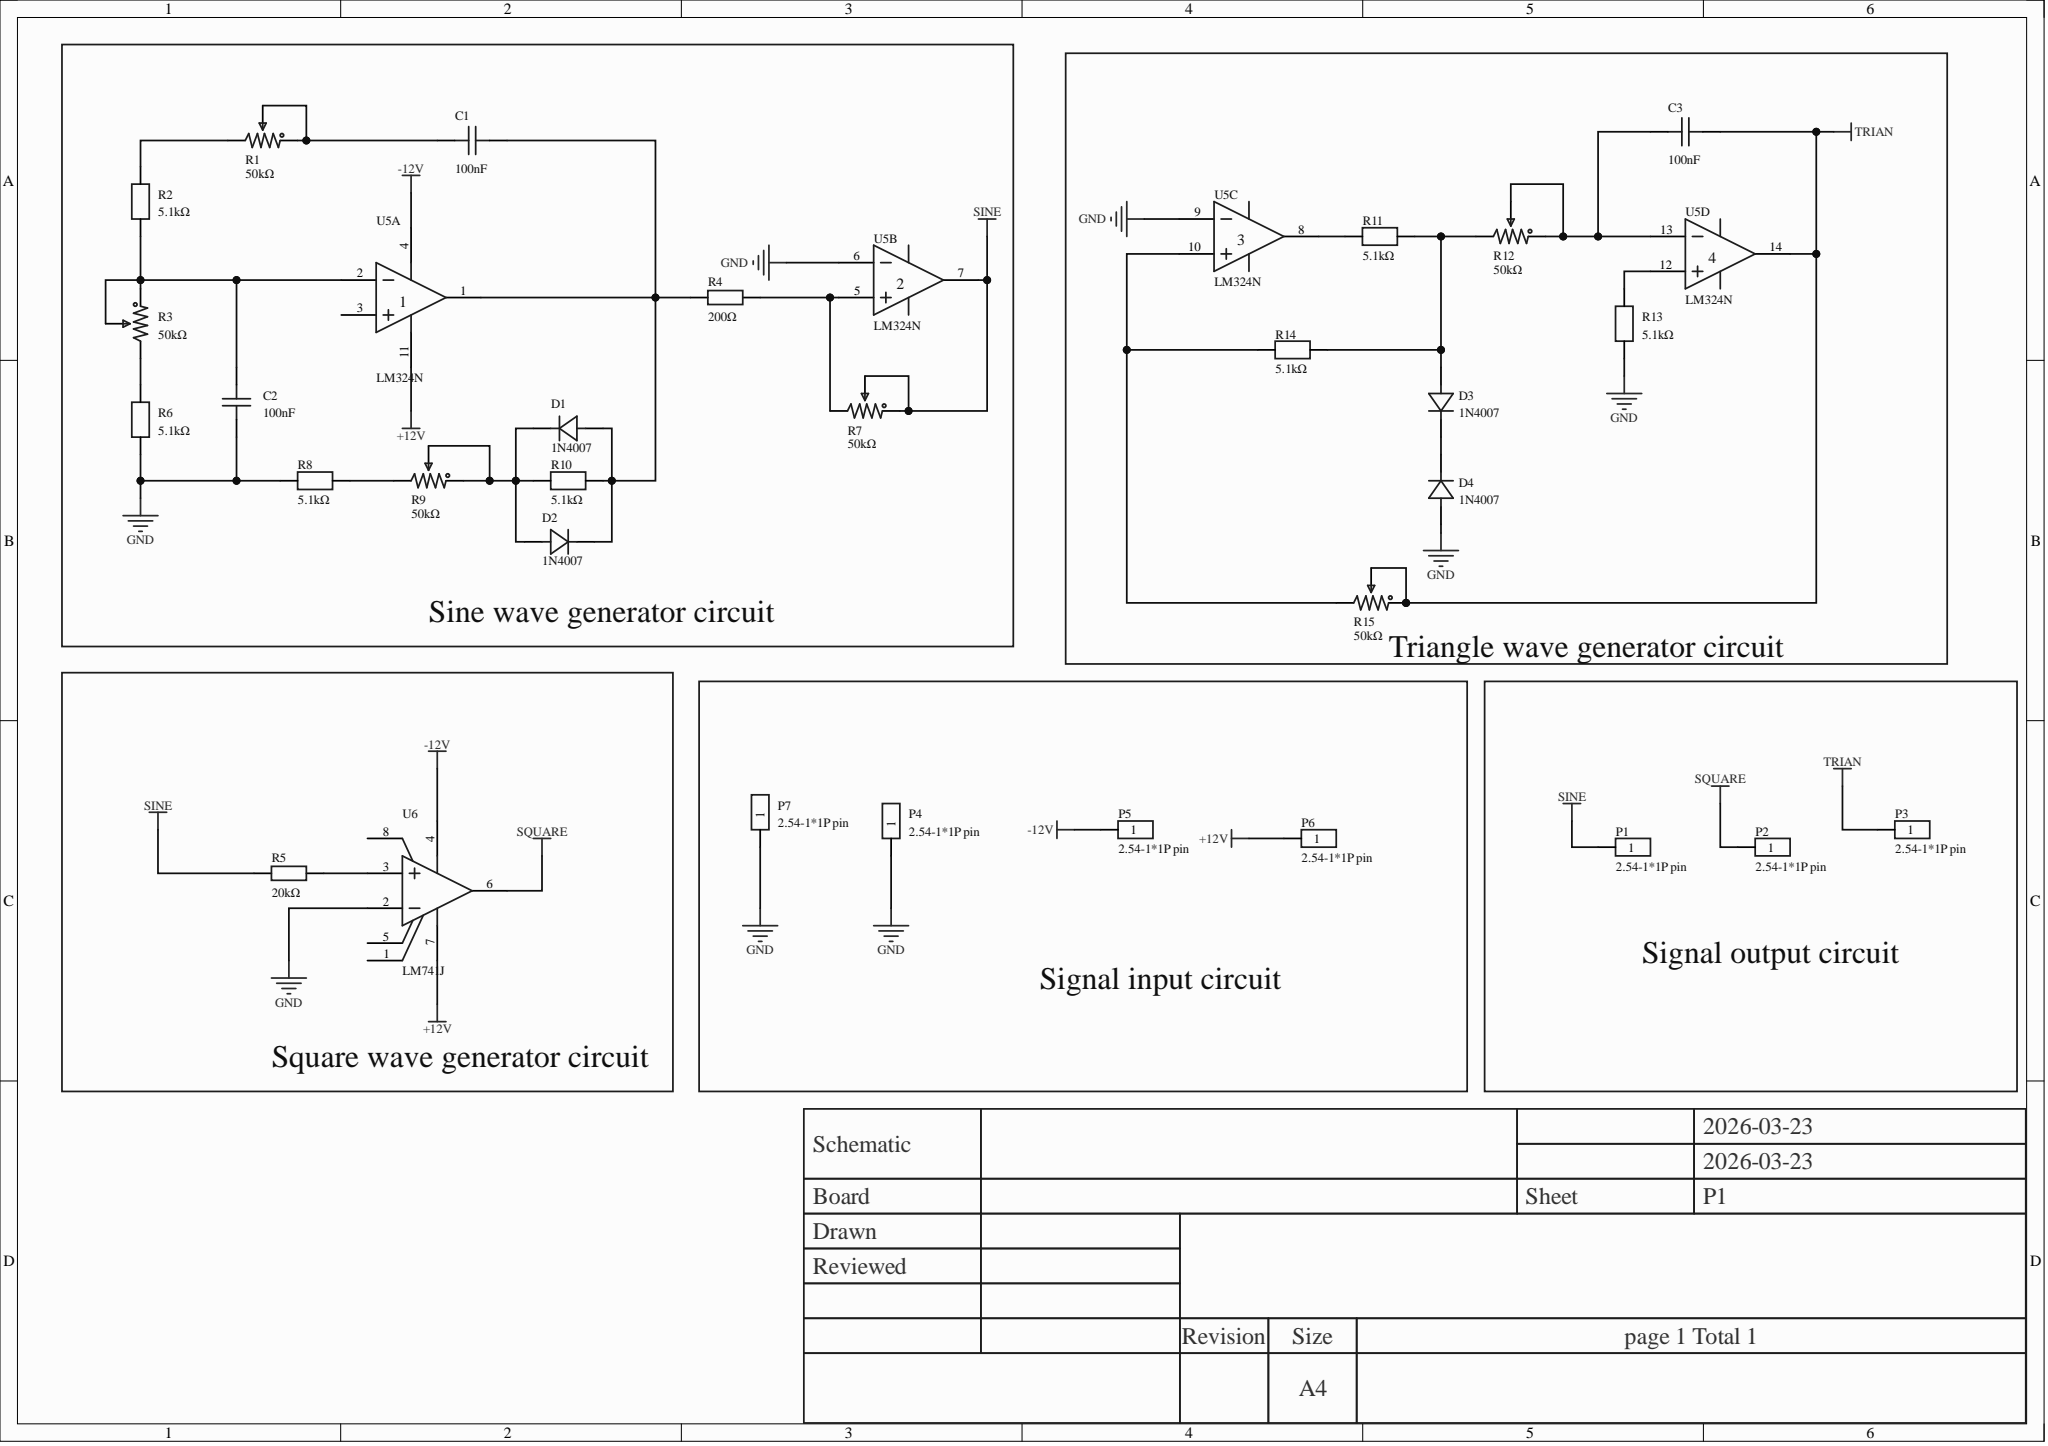Circuit board | Altium Designer | 31 parts | 21 nets
Bill of materials:
Comment,Description,Designator,Footprint,LibRef,Quantity
"100nF","","C1, C2, C3","C0603","CGA0603X7R104K500JT","3"
"1N4007","","D1, D3, D4","SMA_L4.3-W2.5-LS5.0-RD","1N4007_C2985028, 1N4007_C727081","3"
"1N4007","","D2","SMA_L4.3-W2.5-LS5.0-RD-1","1N4007_C2985028","1"
"2.54-1*1P pin","","P1, P2, P3, P4, P5, P6, P7","HDR-TH_1P-P2.54-V-M","2.54-1*1P针","7"
"50kΩ","","R1, R3, R7, R9, R12, R15","RES-ADJ-TH_3P-L9.5-W4.85-P2.50-BL-BS","3296W-1-503_C48997928","6"
"5.1kΩ","","R2, R6, R8, R10, R11, R13, R14","R0603","FRC0603F5101TS","7"
"200Ω","","R4","R0603","0603WAF2000T5E","1"
"20kΩ","","R5","R0603","0603WAF2002T5E","1"
"LM324N","Amplifier count: quad; rail-to-rail: -; gain bandwidth product (GBP): -; input offset voltage (Vos): 9mV; slew rate (SR): -; input bias current (Ib): 250nA;","U5","DIP-14_L19.4-W6.4-P2.54-LS7.6-BL","LM324N_C725320","1"
"LM741J","","U6","CDIP-8_L10.3-W6.7-P2.54-LS7.6-BL","LM741J","1"
Netlist (Protel format):
[
C1
C0603
100nF



]
[
C2
C0603
100nF



]
[
C3
C0603
100nF



]
[
D1
SMA_L4.3-W2.5-LS5.0-RD
1N4007



]
[
D2
SMA_L4.3-W2.5-LS5.0-RD-1
1N4007



]
[
D3
SMA_L4.3-W2.5-LS5.0-RD
1N4007



]
[
D4
SMA_L4.3-W2.5-LS5.0-RD
1N4007



]
[
P1
HDR-TH_1P-P2.54-V-M
2.54-1*1P pin



]
[
P2
HDR-TH_1P-P2.54-V-M
2.54-1*1P pin



]
[
P3
HDR-TH_1P-P2.54-V-M
2.54-1*1P pin



]
[
P4
HDR-TH_1P-P2.54-V-M
2.54-1*1P pin



]
[
P5
HDR-TH_1P-P2.54-V-M
2.54-1*1P pin



]
[
P6
HDR-TH_1P-P2.54-V-M
2.54-1*1P pin



]
[
P7
HDR-TH_1P-P2.54-V-M
2.54-1*1P pin



]
[
R1
RES-ADJ-TH_3P-L9.5-W4.85-P2.50-BL-BS
50kΩ



]
[
R2
R0603
5.1kΩ



]
[
R3
RES-ADJ-TH_3P-L9.5-W4.85-P2.50-BL-BS
50kΩ



]
[
R4
R0603
200Ω



]
[
R5
R0603
20kΩ



]
[
R6
R0603
5.1kΩ



]
[
R7
RES-ADJ-TH_3P-L9.5-W4.85-P2.50-BL-BS
50kΩ



]
[
R8
R0603
5.1kΩ



]
[
R9
RES-ADJ-TH_3P-L9.5-W4.85-P2.50-BL-BS
50kΩ



]
[
R10
R0603
5.1kΩ



]
[
R11
R0603
5.1kΩ



]
[
R12
RES-ADJ-TH_3P-L9.5-W4.85-P2.50-BL-BS
50kΩ



]
[
R13
R0603
5.1kΩ



]
[
R14
R0603
5.1kΩ



]
[
R15
RES-ADJ-TH_3P-L9.5-W4.85-P2.50-BL-BS
50kΩ



]
[
U5
DIP-14_L19.4-W6.4-P2.54-LS7.6-BL
LM324N



]
[
U6
CDIP-8_L10.3-W6.7-P2.54-LS7.6-BL
LM741J



]
(
TRIAN
C3-2
P3-1
R15-1
R15-2
U5-14
)
(
SQUARE
P2-1
U6-6
)
(
SINE
P1-1
R5-1
R7-1
R7-2
U5-7
)
(
NetR14_1
R14-1
R15-3
U5-10
)
(
NetR13_2
R13-2
U5-12
)
(
NetR11_1
R11-1
U5-8
)
(
NetR8_2
R8-2
R9-3
)
(
NetR5_2
R5-2
U6-3
)
(
NetR4_2
R4-2
R7-3
U5-5
)
(
NetR3_3
R3-3
R6-2
)
(
NetR1_3
R1-3
R2-2
)
(
NetD3_2
D3-2
R11-2
R12-3
R14-2
)
(
NetD3_1
D3-1
D4-1
)
(
NetD1_1
D1-1
D2-2
R9-1
R9-2
R10-1
)
(
NetC3_1
C3-1
R12-1
R12-2
U5-13
)
(
NetC2_2
C2-2
R2-1
R3-1
R3-2
U5-2
)
(
NetC1_2
C1-2
D1-2
D2-1
R4-1
R10-2
U5-1
)
(
NetC1_1
C1-1
R1-1
R1-2
)
(
GND
C2-1
D4-2
P4-1
P7-1
R6-1
R8-1
R13-1
U5-6
U5-9
U6-2
)
(
-12V
P5-1
U5-4
U6-4
)
(
+12V
P6-1
U5-11
U6-7
)